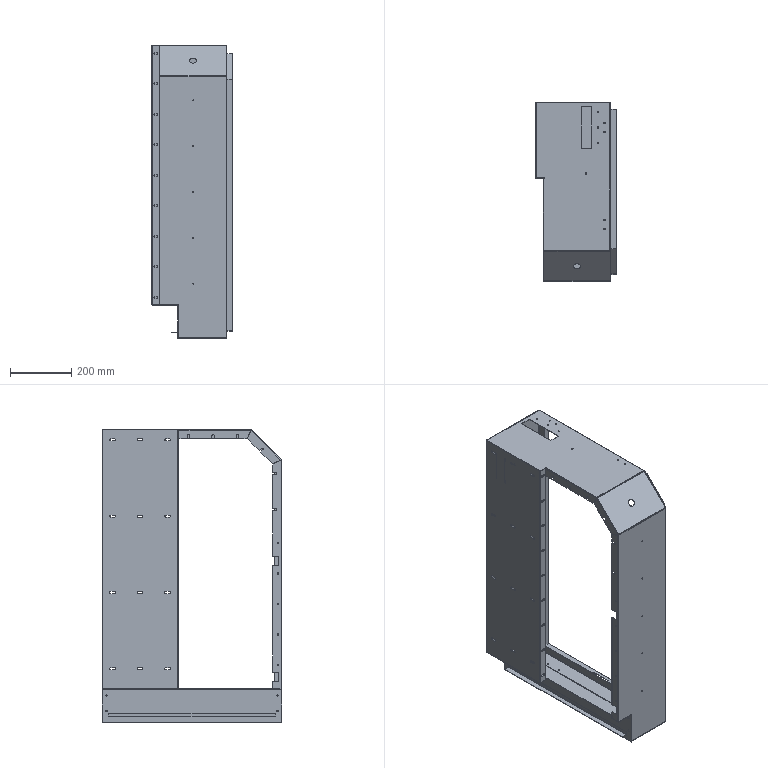Part | SolidWorks | features HoleWzd 16, ICE 8, Cut 6, FlatPattern 6, SheetMetal 6, SolidToSheetMetal 4, SMBaseFlange 3, EdgeFlange 2, MoveFace 2, Chamfer 1, Extrusion 1 | 6 solids | 390 faces | box 264.5 x 588 x 960 mm | volume 1725944 mm3 | plane 223 | cylinder 159 | spline 8 | commonest cylinder face diameters 7 x52 4.2 x34 4.8 x22 1.473 x14 4.473 x13 3.3 x10